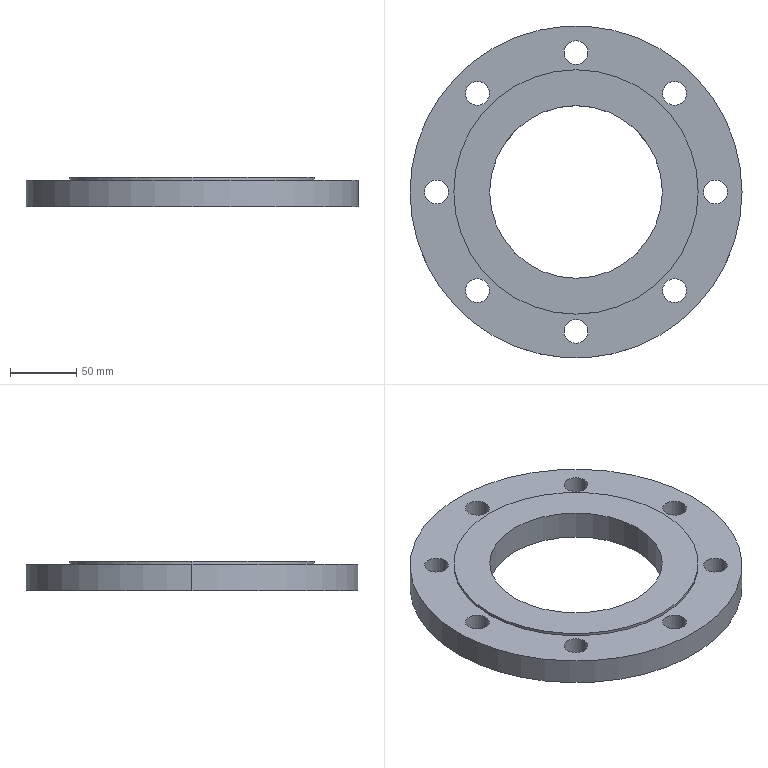Part | SolidWorks | features Extrusion 1, ICE 1 | 1 solid | 25 faces | box 250 x 250 x 22 mm | volume 702203 mm3 | cylinder 22 | plane 3 | commonest cylinder face diameters 18 x16 130 x2 184 x2 250 x2
STEP:
#1=CARTESIAN_POINT('',(92.,0.,22.));
#2=VERTEX_POINT('',#1);
#3=CARTESIAN_POINT('',(-92.,0.,22.));
#4=VERTEX_POINT('',#3);
#5=CARTESIAN_POINT('',(0.,0.,22.));
#6=DIRECTION('',(0.,0.,1.));
#7=DIRECTION('',(1.,0.,0.));
#8=AXIS2_PLACEMENT_3D('',#5,#6,#7);
#9=CIRCLE('',#8,92.);
#10=EDGE_CURVE('',#2,#4,#9,.T.);
#11=ORIENTED_EDGE('',*,*,#10,.F.);
#12=CARTESIAN_POINT('',(92.,0.,20.));
#13=VERTEX_POINT('',#12);
#14=CARTESIAN_POINT('',(92.,0.,22.));
#15=DIRECTION('',(0.,0.,-1.));
#16=VECTOR('',#15,1000.);
#17=LINE('',#14,#16);
#18=EDGE_CURVE('',#2,#13,#17,.T.);
#19=ORIENTED_EDGE('',*,*,#18,.T.);
#20=CARTESIAN_POINT('',(-92.,0.,20.));
#21=VERTEX_POINT('',#20);
#22=CARTESIAN_POINT('',(0.,0.,20.));
#23=DIRECTION('',(0.,0.,1.));
#24=DIRECTION('',(1.,0.,0.));
#25=AXIS2_PLACEMENT_3D('',#22,#23,#24);
#26=CIRCLE('',#25,92.);
#27=EDGE_CURVE('',#13,#21,#26,.T.);
#28=ORIENTED_EDGE('',*,*,#27,.T.);
#29=CARTESIAN_POINT('',(-92.,0.,22.));
#30=DIRECTION('',(0.,0.,-1.));
#31=VECTOR('',#30,1000.);
#32=LINE('',#29,#31);
#33=EDGE_CURVE('',#4,#21,#32,.T.);
#34=ORIENTED_EDGE('',*,*,#33,.F.);
#35=EDGE_LOOP('',(#11,#19,#28,#34));
#36=FACE_OUTER_BOUND('',#35,.T.);
#37=CARTESIAN_POINT('',(0.,0.,22.));
#38=DIRECTION('',(0.,0.,-1.));
#39=DIRECTION('',(-1.,0.,0.));
#40=AXIS2_PLACEMENT_3D('',#37,#38,#39);
#41=CYLINDRICAL_SURFACE('',#40,92.);
#42=ADVANCED_FACE('',(#36),#41,.T.);
#43=CARTESIAN_POINT('',(-83.246,74.246,20.));
#44=VERTEX_POINT('',#43);
#45=CARTESIAN_POINT('',(-65.246,74.246,20.));
#46=VERTEX_POINT('',#45);
#47=CARTESIAN_POINT('',(-74.246,74.246,20.));
#48=DIRECTION('',(0.,0.,1.));
#49=DIRECTION('',(1.,0.,0.));
#50=AXIS2_PLACEMENT_3D('',#47,#48,#49);
#51=CIRCLE('',#50,9.);
#52=EDGE_CURVE('',#44,#46,#51,.T.);
#53=ORIENTED_EDGE('',*,*,#52,.T.);
#54=CARTESIAN_POINT('',(-65.246,74.246,0.));
#55=VERTEX_POINT('',#54);
#56=CARTESIAN_POINT('',(-65.246,74.246,20.));
#57=DIRECTION('',(0.,0.,-1.));
#58=VECTOR('',#57,1000.);
#59=LINE('',#56,#58);
#60=EDGE_CURVE('',#46,#55,#59,.T.);
#61=ORIENTED_EDGE('',*,*,#60,.T.);
#62=CARTESIAN_POINT('',(-83.246,74.246,0.));
#63=VERTEX_POINT('',#62);
#64=CARTESIAN_POINT('',(-74.246,74.246,0.));
#65=DIRECTION('',(0.,0.,1.));
#66=DIRECTION('',(1.,0.,0.));
#67=AXIS2_PLACEMENT_3D('',#64,#65,#66);
#68=CIRCLE('',#67,9.);
#69=EDGE_CURVE('',#63,#55,#68,.T.);
#70=ORIENTED_EDGE('',*,*,#69,.F.);
#71=CARTESIAN_POINT('',(-83.246,74.246,20.));
#72=DIRECTION('',(0.,0.,-1.));
#73=VECTOR('',#72,1000.);
#74=LINE('',#71,#73);
#75=EDGE_CURVE('',#44,#63,#74,.T.);
#76=ORIENTED_EDGE('',*,*,#75,.F.);
#77=EDGE_LOOP('',(#53,#61,#70,#76));
#78=FACE_OUTER_BOUND('',#77,.T.);
#79=CARTESIAN_POINT('',(-74.246,74.246,20.));
#80=DIRECTION('',(0.,0.,-1.));
#81=DIRECTION('',(-1.,0.,0.));
#82=AXIS2_PLACEMENT_3D('',#79,#80,#81);
#83=CYLINDRICAL_SURFACE('',#82,9.);
#84=ADVANCED_FACE('',(#78),#83,.F.);
#85=CARTESIAN_POINT('',(-114.,0.,20.));
#86=VERTEX_POINT('',#85);
#87=CARTESIAN_POINT('',(-96.,0.,20.));
#88=VERTEX_POINT('',#87);
#89=CARTESIAN_POINT('',(-105.,0.,20.));
#90=DIRECTION('',(0.,0.,1.));
#91=DIRECTION('',(1.,0.,0.));
#92=AXIS2_PLACEMENT_3D('',#89,#90,#91);
#93=CIRCLE('',#92,9.);
#94=EDGE_CURVE('',#86,#88,#93,.T.);
#95=ORIENTED_EDGE('',*,*,#94,.T.);
#96=CARTESIAN_POINT('',(-96.,0.,0.));
#97=VERTEX_POINT('',#96);
#98=CARTESIAN_POINT('',(-96.,0.,20.));
#99=DIRECTION('',(0.,0.,-1.));
#100=VECTOR('',#99,1000.);
#101=LINE('',#98,#100);
#102=EDGE_CURVE('',#88,#97,#101,.T.);
#103=ORIENTED_EDGE('',*,*,#102,.T.);
#104=CARTESIAN_POINT('',(-114.,0.,0.));
#105=VERTEX_POINT('',#104);
#106=CARTESIAN_POINT('',(-105.,0.,0.));
#107=DIRECTION('',(0.,0.,1.));
#108=DIRECTION('',(1.,0.,0.));
#109=AXIS2_PLACEMENT_3D('',#106,#107,#108);
#110=CIRCLE('',#109,9.);
#111=EDGE_CURVE('',#105,#97,#110,.T.);
#112=ORIENTED_EDGE('',*,*,#111,.F.);
#113=CARTESIAN_POINT('',(-114.,0.,20.));
#114=DIRECTION('',(0.,0.,-1.));
#115=VECTOR('',#114,1000.);
#116=LINE('',#113,#115);
#117=EDGE_CURVE('',#86,#105,#116,.T.);
#118=ORIENTED_EDGE('',*,*,#117,.F.);
#119=EDGE_LOOP('',(#95,#103,#112,#118));
#120=FACE_OUTER_BOUND('',#119,.T.);
#121=CARTESIAN_POINT('',(-105.,0.,20.));
#122=DIRECTION('',(0.,0.,-1.));
#123=DIRECTION('',(-1.,0.,0.));
#124=AXIS2_PLACEMENT_3D('',#121,#122,#123);
#125=CYLINDRICAL_SURFACE('',#124,9.);
#126=ADVANCED_FACE('',(#120),#125,.F.);
#127=CARTESIAN_POINT('',(-83.246,-74.246,20.));
#128=VERTEX_POINT('',#127);
#129=CARTESIAN_POINT('',(-65.246,-74.246,20.));
#130=VERTEX_POINT('',#129);
#131=CARTESIAN_POINT('',(-74.246,-74.246,20.));
#132=DIRECTION('',(0.,0.,1.));
#133=DIRECTION('',(1.,0.,0.));
#134=AXIS2_PLACEMENT_3D('',#131,#132,#133);
#135=CIRCLE('',#134,9.);
#136=EDGE_CURVE('',#128,#130,#135,.T.);
#137=ORIENTED_EDGE('',*,*,#136,.T.);
#138=CARTESIAN_POINT('',(-65.246,-74.246,0.));
#139=VERTEX_POINT('',#138);
#140=CARTESIAN_POINT('',(-65.246,-74.246,20.));
#141=DIRECTION('',(0.,0.,-1.));
#142=VECTOR('',#141,1000.);
#143=LINE('',#140,#142);
#144=EDGE_CURVE('',#130,#139,#143,.T.);
#145=ORIENTED_EDGE('',*,*,#144,.T.);
#146=CARTESIAN_POINT('',(-83.246,-74.246,0.));
#147=VERTEX_POINT('',#146);
#148=CARTESIAN_POINT('',(-74.246,-74.246,0.));
#149=DIRECTION('',(0.,0.,1.));
#150=DIRECTION('',(1.,0.,0.));
#151=AXIS2_PLACEMENT_3D('',#148,#149,#150);
#152=CIRCLE('',#151,9.);
#153=EDGE_CURVE('',#147,#139,#152,.T.);
#154=ORIENTED_EDGE('',*,*,#153,.F.);
#155=CARTESIAN_POINT('',(-83.246,-74.246,20.));
#156=DIRECTION('',(0.,0.,-1.));
#157=VECTOR('',#156,1000.);
#158=LINE('',#155,#157);
#159=EDGE_CURVE('',#128,#147,#158,.T.);
#160=ORIENTED_EDGE('',*,*,#159,.F.);
#161=EDGE_LOOP('',(#137,#145,#154,#160));
#162=FACE_OUTER_BOUND('',#161,.T.);
#163=CARTESIAN_POINT('',(-74.246,-74.246,20.));
#164=DIRECTION('',(0.,0.,-1.));
#165=DIRECTION('',(-1.,0.,0.));
#166=AXIS2_PLACEMENT_3D('',#163,#164,#165);
#167=CYLINDRICAL_SURFACE('',#166,9.);
#168=ADVANCED_FACE('',(#162),#167,.F.);
#169=CARTESIAN_POINT('',(-9.,-105.,20.));
#170=VERTEX_POINT('',#169);
#171=CARTESIAN_POINT('',(9.,-105.,20.));
#172=VERTEX_POINT('',#171);
#173=CARTESIAN_POINT('',(0.,-105.,20.));
#174=DIRECTION('',(0.,0.,1.));
#175=DIRECTION('',(1.,0.,0.));
#176=AXIS2_PLACEMENT_3D('',#173,#174,#175);
#177=CIRCLE('',#176,9.);
#178=EDGE_CURVE('',#170,#172,#177,.T.);
#179=ORIENTED_EDGE('',*,*,#178,.T.);
#180=CARTESIAN_POINT('',(9.,-105.,0.));
#181=VERTEX_POINT('',#180);
#182=CARTESIAN_POINT('',(9.,-105.,20.));
#183=DIRECTION('',(0.,0.,-1.));
#184=VECTOR('',#183,1000.);
#185=LINE('',#182,#184);
#186=EDGE_CURVE('',#172,#181,#185,.T.);
#187=ORIENTED_EDGE('',*,*,#186,.T.);
#188=CARTESIAN_POINT('',(-9.,-105.,0.));
#189=VERTEX_POINT('',#188);
#190=CARTESIAN_POINT('',(0.,-105.,0.));
#191=DIRECTION('',(0.,0.,1.));
#192=DIRECTION('',(1.,0.,0.));
#193=AXIS2_PLACEMENT_3D('',#190,#191,#192);
#194=CIRCLE('',#193,9.);
#195=EDGE_CURVE('',#189,#181,#194,.T.);
#196=ORIENTED_EDGE('',*,*,#195,.F.);
#197=CARTESIAN_POINT('',(-9.,-105.,20.));
#198=DIRECTION('',(0.,0.,-1.));
#199=VECTOR('',#198,1000.);
#200=LINE('',#197,#199);
#201=EDGE_CURVE('',#170,#189,#200,.T.);
#202=ORIENTED_EDGE('',*,*,#201,.F.);
#203=EDGE_LOOP('',(#179,#187,#196,#202));
#204=FACE_OUTER_BOUND('',#203,.T.);
#205=CARTESIAN_POINT('',(0.,-105.,20.));
#206=DIRECTION('',(0.,0.,-1.));
#207=DIRECTION('',(-1.,0.,0.));
#208=AXIS2_PLACEMENT_3D('',#205,#206,#207);
#209=CYLINDRICAL_SURFACE('',#208,9.);
#210=ADVANCED_FACE('',(#204),#209,.F.);
#211=CARTESIAN_POINT('',(65.246,-74.246,20.));
#212=VERTEX_POINT('',#211);
#213=CARTESIAN_POINT('',(83.246,-74.246,20.));
#214=VERTEX_POINT('',#213);
#215=CARTESIAN_POINT('',(74.246,-74.246,20.));
#216=DIRECTION('',(0.,0.,1.));
#217=DIRECTION('',(1.,0.,0.));
#218=AXIS2_PLACEMENT_3D('',#215,#216,#217);
#219=CIRCLE('',#218,9.);
#220=EDGE_CURVE('',#212,#214,#219,.T.);
#221=ORIENTED_EDGE('',*,*,#220,.T.);
#222=CARTESIAN_POINT('',(83.246,-74.246,0.));
#223=VERTEX_POINT('',#222);
#224=CARTESIAN_POINT('',(83.246,-74.246,20.));
#225=DIRECTION('',(0.,0.,-1.));
#226=VECTOR('',#225,1000.);
#227=LINE('',#224,#226);
#228=EDGE_CURVE('',#214,#223,#227,.T.);
#229=ORIENTED_EDGE('',*,*,#228,.T.);
#230=CARTESIAN_POINT('',(65.246,-74.246,0.));
#231=VERTEX_POINT('',#230);
#232=CARTESIAN_POINT('',(74.246,-74.246,0.));
#233=DIRECTION('',(0.,0.,1.));
#234=DIRECTION('',(1.,0.,0.));
#235=AXIS2_PLACEMENT_3D('',#232,#233,#234);
#236=CIRCLE('',#235,9.);
#237=EDGE_CURVE('',#231,#223,#236,.T.);
#238=ORIENTED_EDGE('',*,*,#237,.F.);
#239=CARTESIAN_POINT('',(65.246,-74.246,20.));
#240=DIRECTION('',(0.,0.,-1.));
#241=VECTOR('',#240,1000.);
#242=LINE('',#239,#241);
#243=EDGE_CURVE('',#212,#231,#242,.T.);
#244=ORIENTED_EDGE('',*,*,#243,.F.);
#245=EDGE_LOOP('',(#221,#229,#238,#244));
#246=FACE_OUTER_BOUND('',#245,.T.);
#247=CARTESIAN_POINT('',(74.246,-74.246,20.));
#248=DIRECTION('',(0.,0.,-1.));
#249=DIRECTION('',(-1.,0.,0.));
#250=AXIS2_PLACEMENT_3D('',#247,#248,#249);
#251=CYLINDRICAL_SURFACE('',#250,9.);
#252=ADVANCED_FACE('',(#246),#251,.F.);
#253=CARTESIAN_POINT('',(96.,0.,20.));
#254=VERTEX_POINT('',#253);
#255=CARTESIAN_POINT('',(114.,0.,20.));
#256=VERTEX_POINT('',#255);
#257=CARTESIAN_POINT('',(105.,0.,20.));
#258=DIRECTION('',(0.,0.,1.));
#259=DIRECTION('',(1.,0.,0.));
#260=AXIS2_PLACEMENT_3D('',#257,#258,#259);
#261=CIRCLE('',#260,9.);
#262=EDGE_CURVE('',#254,#256,#261,.T.);
#263=ORIENTED_EDGE('',*,*,#262,.T.);
#264=CARTESIAN_POINT('',(114.,0.,0.));
#265=VERTEX_POINT('',#264);
#266=CARTESIAN_POINT('',(114.,0.,20.));
#267=DIRECTION('',(0.,0.,-1.));
#268=VECTOR('',#267,1000.);
#269=LINE('',#266,#268);
#270=EDGE_CURVE('',#256,#265,#269,.T.);
#271=ORIENTED_EDGE('',*,*,#270,.T.);
#272=CARTESIAN_POINT('',(96.,0.,0.));
#273=VERTEX_POINT('',#272);
#274=CARTESIAN_POINT('',(105.,0.,0.));
#275=DIRECTION('',(0.,0.,1.));
#276=DIRECTION('',(1.,0.,0.));
#277=AXIS2_PLACEMENT_3D('',#274,#275,#276);
#278=CIRCLE('',#277,9.);
#279=EDGE_CURVE('',#273,#265,#278,.T.);
#280=ORIENTED_EDGE('',*,*,#279,.F.);
#281=CARTESIAN_POINT('',(96.,0.,20.));
#282=DIRECTION('',(0.,0.,-1.));
#283=VECTOR('',#282,1000.);
#284=LINE('',#281,#283);
#285=EDGE_CURVE('',#254,#273,#284,.T.);
#286=ORIENTED_EDGE('',*,*,#285,.F.);
#287=EDGE_LOOP('',(#263,#271,#280,#286));
#288=FACE_OUTER_BOUND('',#287,.T.);
#289=CARTESIAN_POINT('',(105.,0.,20.));
#290=DIRECTION('',(0.,0.,-1.));
#291=DIRECTION('',(-1.,0.,0.));
#292=AXIS2_PLACEMENT_3D('',#289,#290,#291);
#293=CYLINDRICAL_SURFACE('',#292,9.);
#294=ADVANCED_FACE('',(#288),#293,.F.);
#295=CARTESIAN_POINT('',(65.246,74.246,20.));
#296=VERTEX_POINT('',#295);
#297=CARTESIAN_POINT('',(83.246,74.246,20.));
#298=VERTEX_POINT('',#297);
#299=CARTESIAN_POINT('',(74.246,74.246,20.));
#300=DIRECTION('',(0.,0.,1.));
#301=DIRECTION('',(1.,0.,0.));
#302=AXIS2_PLACEMENT_3D('',#299,#300,#301);
#303=CIRCLE('',#302,9.);
#304=EDGE_CURVE('',#296,#298,#303,.T.);
#305=ORIENTED_EDGE('',*,*,#304,.T.);
#306=CARTESIAN_POINT('',(83.246,74.246,0.));
#307=VERTEX_POINT('',#306);
#308=CARTESIAN_POINT('',(83.246,74.246,20.));
#309=DIRECTION('',(0.,0.,-1.));
#310=VECTOR('',#309,1000.);
#311=LINE('',#308,#310);
#312=EDGE_CURVE('',#298,#307,#311,.T.);
#313=ORIENTED_EDGE('',*,*,#312,.T.);
#314=CARTESIAN_POINT('',(65.246,74.246,0.));
#315=VERTEX_POINT('',#314);
#316=CARTESIAN_POINT('',(74.246,74.246,0.));
#317=DIRECTION('',(0.,0.,1.));
#318=DIRECTION('',(1.,0.,0.));
#319=AXIS2_PLACEMENT_3D('',#316,#317,#318);
#320=CIRCLE('',#319,9.);
#321=EDGE_CURVE('',#315,#307,#320,.T.);
#322=ORIENTED_EDGE('',*,*,#321,.F.);
#323=CARTESIAN_POINT('',(65.246,74.246,20.));
#324=DIRECTION('',(0.,0.,-1.));
#325=VECTOR('',#324,1000.);
#326=LINE('',#323,#325);
#327=EDGE_CURVE('',#296,#315,#326,.T.);
#328=ORIENTED_EDGE('',*,*,#327,.F.);
#329=EDGE_LOOP('',(#305,#313,#322,#328));
#330=FACE_OUTER_BOUND('',#329,.T.);
#331=CARTESIAN_POINT('',(74.246,74.246,20.));
#332=DIRECTION('',(0.,0.,-1.));
#333=DIRECTION('',(-1.,0.,0.));
#334=AXIS2_PLACEMENT_3D('',#331,#332,#333);
#335=CYLINDRICAL_SURFACE('',#334,9.);
#336=ADVANCED_FACE('',(#330),#335,.F.);
#337=CARTESIAN_POINT('',(-9.,105.,20.));
#338=VERTEX_POINT('',#337);
#339=CARTESIAN_POINT('',(9.,105.,20.));
#340=VERTEX_POINT('',#339);
#341=CARTESIAN_POINT('',(0.,105.,20.));
#342=DIRECTION('',(0.,0.,1.));
#343=DIRECTION('',(1.,0.,0.));
#344=AXIS2_PLACEMENT_3D('',#341,#342,#343);
#345=CIRCLE('',#344,9.);
#346=EDGE_CURVE('',#338,#340,#345,.T.);
#347=ORIENTED_EDGE('',*,*,#346,.T.);
#348=CARTESIAN_POINT('',(9.,105.,0.));
#349=VERTEX_POINT('',#348);
#350=CARTESIAN_POINT('',(9.,105.,20.));
#351=DIRECTION('',(0.,0.,-1.));
#352=VECTOR('',#351,1000.);
#353=LINE('',#350,#352);
#354=EDGE_CURVE('',#340,#349,#353,.T.);
#355=ORIENTED_EDGE('',*,*,#354,.T.);
#356=CARTESIAN_POINT('',(-9.,105.,0.));
#357=VERTEX_POINT('',#356);
#358=CARTESIAN_POINT('',(0.,105.,0.));
#359=DIRECTION('',(0.,0.,1.));
#360=DIRECTION('',(1.,0.,0.));
#361=AXIS2_PLACEMENT_3D('',#358,#359,#360);
#362=CIRCLE('',#361,9.);
#363=EDGE_CURVE('',#357,#349,#362,.T.);
#364=ORIENTED_EDGE('',*,*,#363,.F.);
#365=CARTESIAN_POINT('',(-9.,105.,20.));
#366=DIRECTION('',(0.,0.,-1.));
#367=VECTOR('',#366,1000.);
#368=LINE('',#365,#367);
#369=EDGE_CURVE('',#338,#357,#368,.T.);
#370=ORIENTED_EDGE('',*,*,#369,.F.);
#371=EDGE_LOOP('',(#347,#355,#364,#370));
#372=FACE_OUTER_BOUND('',#371,.T.);
#373=CARTESIAN_POINT('',(0.,105.,20.));
#374=DIRECTION('',(0.,0.,-1.));
#375=DIRECTION('',(-1.,0.,0.));
#376=AXIS2_PLACEMENT_3D('',#373,#374,#375);
#377=CYLINDRICAL_SURFACE('',#376,9.);
#378=ADVANCED_FACE('',(#372),#377,.F.);
#379=CARTESIAN_POINT('',(-65.,0.,22.));
#380=VERTEX_POINT('',#379);
#381=CARTESIAN_POINT('',(65.,0.,22.));
#382=VERTEX_POINT('',#381);
#383=CARTESIAN_POINT('',(0.,0.,22.));
#384=DIRECTION('',(0.,0.,1.));
#385=DIRECTION('',(1.,0.,0.));
#386=AXIS2_PLACEMENT_3D('',#383,#384,#385);
#387=CIRCLE('',#386,65.);
#388=EDGE_CURVE('',#380,#382,#387,.T.);
#389=ORIENTED_EDGE('',*,*,#388,.T.);
#390=CARTESIAN_POINT('',(65.,0.,0.));
#391=VERTEX_POINT('',#390);
#392=CARTESIAN_POINT('',(65.,0.,20.));
#393=DIRECTION('',(0.,0.,-1.));
#394=VECTOR('',#393,1000.);
#395=LINE('',#392,#394);
#396=EDGE_CURVE('',#382,#391,#395,.T.);
#397=ORIENTED_EDGE('',*,*,#396,.T.);
#398=CARTESIAN_POINT('',(-65.,0.,0.));
#399=VERTEX_POINT('',#398);
#400=CARTESIAN_POINT('',(0.,0.,0.));
#401=DIRECTION('',(0.,0.,1.));
#402=DIRECTION('',(1.,0.,0.));
#403=AXIS2_PLACEMENT_3D('',#400,#401,#402);
#404=CIRCLE('',#403,65.);
#405=EDGE_CURVE('',#399,#391,#404,.T.);
#406=ORIENTED_EDGE('',*,*,#405,.F.);
#407=CARTESIAN_POINT('',(-65.,0.,20.));
#408=DIRECTION('',(0.,0.,-1.));
#409=VECTOR('',#408,1000.);
#410=LINE('',#407,#409);
#411=EDGE_CURVE('',#380,#399,#410,.T.);
#412=ORIENTED_EDGE('',*,*,#411,.F.);
#413=EDGE_LOOP('',(#389,#397,#406,#412));
#414=FACE_OUTER_BOUND('',#413,.T.);
#415=CARTESIAN_POINT('',(0.,0.,20.));
#416=DIRECTION('',(0.,0.,-1.));
#417=DIRECTION('',(-1.,0.,0.));
#418=AXIS2_PLACEMENT_3D('',#415,#416,#417);
#419=CYLINDRICAL_SURFACE('',#418,65.);
#420=ADVANCED_FACE('',(#414),#419,.F.);
#421=CARTESIAN_POINT('',(125.,0.,20.));
#422=VERTEX_POINT('',#421);
#423=CARTESIAN_POINT('',(-125.,0.,20.));
#424=VERTEX_POINT('',#423);
#425=CARTESIAN_POINT('',(0.,0.,20.));
#426=DIRECTION('',(0.,0.,1.));
#427=DIRECTION('',(1.,0.,0.));
#428=AXIS2_PLACEMENT_3D('',#425,#426,#427);
#429=CIRCLE('',#428,125.);
#430=EDGE_CURVE('',#422,#424,#429,.T.);
#431=ORIENTED_EDGE('',*,*,#430,.F.);
#432=CARTESIAN_POINT('',(125.,0.,0.));
#433=VERTEX_POINT('',#432);
#434=CARTESIAN_POINT('',(125.,0.,20.));
#435=DIRECTION('',(0.,0.,-1.));
#436=VECTOR('',#435,1000.);
#437=LINE('',#434,#436);
#438=EDGE_CURVE('',#422,#433,#437,.T.);
#439=ORIENTED_EDGE('',*,*,#438,.T.);
#440=CARTESIAN_POINT('',(-125.,0.,0.));
#441=VERTEX_POINT('',#440);
#442=CARTESIAN_POINT('',(0.,0.,0.));
#443=DIRECTION('',(0.,0.,1.));
#444=DIRECTION('',(1.,0.,0.));
#445=AXIS2_PLACEMENT_3D('',#442,#443,#444);
#446=CIRCLE('',#445,125.);
#447=EDGE_CURVE('',#433,#441,#446,.T.);
#448=ORIENTED_EDGE('',*,*,#447,.T.);
#449=CARTESIAN_POINT('',(-125.,0.,20.));
#450=DIRECTION('',(0.,0.,-1.));
#451=VECTOR('',#450,1000.);
#452=LINE('',#449,#451);
#453=EDGE_CURVE('',#424,#441,#452,.T.);
#454=ORIENTED_EDGE('',*,*,#453,.F.);
#455=EDGE_LOOP('',(#431,#439,#448,#454));
#456=FACE_OUTER_BOUND('',#455,.T.);
#457=CARTESIAN_POINT('',(0.,0.,20.));
#458=DIRECTION('',(0.,0.,-1.));
#459=DIRECTION('',(-1.,0.,0.));
#460=AXIS2_PLACEMENT_3D('',#457,#458,#459);
#461=CYLINDRICAL_SURFACE('',#460,125.);
#462=ADVANCED_FACE('',(#456),#461,.T.);
#463=ORIENTED_EDGE('',*,*,#52,.F.);
#464=CARTESIAN_POINT('',(-74.246,74.246,20.));
#465=DIRECTION('',(0.,0.,1.));
#466=DIRECTION('',(1.,0.,0.));
#467=AXIS2_PLACEMENT_3D('',#464,#465,#466);
#468=CIRCLE('',#467,9.);
#469=EDGE_CURVE('',#46,#44,#468,.T.);
#470=ORIENTED_EDGE('',*,*,#469,.F.);
#471=EDGE_LOOP('',(#463,#470));
#472=FACE_BOUND('',#471,.T.);
#473=ORIENTED_EDGE('',*,*,#136,.F.);
#474=CARTESIAN_POINT('',(-74.246,-74.246,20.));
#475=DIRECTION('',(0.,0.,1.));
#476=DIRECTION('',(1.,0.,0.));
#477=AXIS2_PLACEMENT_3D('',#474,#475,#476);
#478=CIRCLE('',#477,9.);
#479=EDGE_CURVE('',#130,#128,#478,.T.);
#480=ORIENTED_EDGE('',*,*,#479,.F.);
#481=EDGE_LOOP('',(#473,#480));
#482=FACE_BOUND('',#481,.T.);
#483=ORIENTED_EDGE('',*,*,#220,.F.);
#484=CARTESIAN_POINT('',(74.246,-74.246,20.));
#485=DIRECTION('',(0.,0.,1.));
#486=DIRECTION('',(1.,0.,0.));
#487=AXIS2_PLACEMENT_3D('',#484,#485,#486);
#488=CIRCLE('',#487,9.);
#489=EDGE_CURVE('',#214,#212,#488,.T.);
#490=ORIENTED_EDGE('',*,*,#489,.F.);
#491=EDGE_LOOP('',(#483,#490));
#492=FACE_BOUND('',#491,.T.);
#493=ORIENTED_EDGE('',*,*,#304,.F.);
#494=CARTESIAN_POINT('',(74.246,74.246,20.));
#495=DIRECTION('',(0.,0.,1.));
#496=DIRECTION('',(1.,0.,0.));
#497=AXIS2_PLACEMENT_3D('',#494,#495,#496);
#498=CIRCLE('',#497,9.);
#499=EDGE_CURVE('',#298,#296,#498,.T.);
#500=ORIENTED_EDGE('',*,*,#499,.F.);
#501=EDGE_LOOP('',(#493,#500));
#502=FACE_BOUND('',#501,.T.);
#503=CARTESIAN_POINT('',(0.,0.,20.));
#504=DIRECTION('',(0.,0.,1.));
#505=DIRECTION('',(1.,0.,0.));
#506=AXIS2_PLACEMENT_3D('',#503,#504,#505);
#507=CIRCLE('',#506,125.);
#508=EDGE_CURVE('',#424,#422,#507,.T.);
#509=ORIENTED_EDGE('',*,*,#508,.T.);
#510=ORIENTED_EDGE('',*,*,#430,.T.);
#511=EDGE_LOOP('',(#509,#510));
#512=FACE_OUTER_BOUND('',#511,.T.);
#513=ORIENTED_EDGE('',*,*,#346,.F.);
#514=CARTESIAN_POINT('',(0.,105.,20.));
#515=DIRECTION('',(0.,0.,1.));
#516=DIRECTION('',(1.,0.,0.));
#517=AXIS2_PLACEMENT_3D('',#514,#515,#516);
#518=CIRCLE('',#517,9.);
#519=EDGE_CURVE('',#340,#338,#518,.T.);
#520=ORIENTED_EDGE('',*,*,#519,.F.);
#521=EDGE_LOOP('',(#513,#520));
#522=FACE_BOUND('',#521,.T.);
#523=ORIENTED_EDGE('',*,*,#262,.F.);
#524=CARTESIAN_POINT('',(105.,0.,20.));
#525=DIRECTION('',(0.,0.,1.));
#526=DIRECTION('',(1.,0.,0.));
#527=AXIS2_PLACEMENT_3D('',#524,#525,#526);
#528=CIRCLE('',#527,9.);
#529=EDGE_CURVE('',#256,#254,#528,.T.);
#530=ORIENTED_EDGE('',*,*,#529,.F.);
#531=EDGE_LOOP('',(#523,#530));
#532=FACE_BOUND('',#531,.T.);
#533=ORIENTED_EDGE('',*,*,#178,.F.);
#534=CARTESIAN_POINT('',(0.,-105.,20.));
#535=DIRECTION('',(0.,0.,1.));
#536=DIRECTION('',(1.,0.,0.));
#537=AXIS2_PLACEMENT_3D('',#534,#535,#536);
#538=CIRCLE('',#537,9.);
#539=EDGE_CURVE('',#172,#170,#538,.T.);
#540=ORIENTED_EDGE('',*,*,#539,.F.);
#541=EDGE_LOOP('',(#533,#540));
#542=FACE_BOUND('',#541,.T.);
#543=ORIENTED_EDGE('',*,*,#94,.F.);
#544=CARTESIAN_POINT('',(-105.,0.,20.));
#545=DIRECTION('',(0.,0.,1.));
#546=DIRECTION('',(1.,0.,0.));
#547=AXIS2_PLACEMENT_3D('',#544,#545,#546);
#548=CIRCLE('',#547,9.);
#549=EDGE_CURVE('',#88,#86,#548,.T.);
#550=ORIENTED_EDGE('',*,*,#549,.F.);
#551=EDGE_LOOP('',(#543,#550));
#552=FACE_BOUND('',#551,.T.);
#553=CARTESIAN_POINT('',(0.,0.,20.));
#554=DIRECTION('',(0.,0.,1.));
#555=DIRECTION('',(1.,0.,0.));
#556=AXIS2_PLACEMENT_3D('',#553,#554,#555);
#557=CIRCLE('',#556,92.);
#558=EDGE_CURVE('',#21,#13,#557,.T.);
#559=ORIENTED_EDGE('',*,*,#558,.F.);
#560=ORIENTED_EDGE('',*,*,#27,.F.);
#561=EDGE_LOOP('',(#559,#560));
#562=FACE_BOUND('',#561,.T.);
#563=CARTESIAN_POINT('',(0.,0.,20.));
#564=DIRECTION('',(0.,0.,1.));
#565=DIRECTION('',(1.,0.,0.));
#566=AXIS2_PLACEMENT_3D('',#563,#564,#565);
#567=PLANE('',#566);
#568=ADVANCED_FACE('',(#472,#482,#492,#502,#512,#522,#532,#542,#552,#562),#567,.T.);
#569=CARTESIAN_POINT('',(0.,0.,0.));
#570=DIRECTION('',(0.,0.,1.));
#571=DIRECTION('',(1.,0.,0.));
#572=AXIS2_PLACEMENT_3D('',#569,#570,#571);
#573=CIRCLE('',#572,125.);
#574=EDGE_CURVE('',#441,#433,#573,.T.);
#575=ORIENTED_EDGE('',*,*,#574,.F.);
#576=ORIENTED_EDGE('',*,*,#447,.F.);
#577=EDGE_LOOP('',(#575,#576));
#578=FACE_OUTER_BOUND('',#577,.T.);
#579=ORIENTED_EDGE('',*,*,#405,.T.);
#580=CARTESIAN_POINT('',(0.,0.,0.));
#581=DIRECTION('',(0.,0.,1.));
#582=DIRECTION('',(1.,0.,0.));
#583=AXIS2_PLACEMENT_3D('',#580,#581,#582);
#584=CIRCLE('',#583,65.);
#585=EDGE_CURVE('',#391,#399,#584,.T.);
#586=ORIENTED_EDGE('',*,*,#585,.T.);
#587=EDGE_LOOP('',(#579,#586));
#588=FACE_BOUND('',#587,.T.);
#589=ORIENTED_EDGE('',*,*,#363,.T.);
#590=CARTESIAN_POINT('',(0.,105.,0.));
#591=DIRECTION('',(0.,0.,1.));
#592=DIRECTION('',(1.,0.,0.));
#593=AXIS2_PLACEMENT_3D('',#590,#591,#592);
#594=CIRCLE('',#593,9.);
#595=EDGE_CURVE('',#349,#357,#594,.T.);
#596=ORIENTED_EDGE('',*,*,#595,.T.);
#597=EDGE_LOOP('',(#589,#596));
#598=FACE_BOUND('',#597,.T.);
#599=ORIENTED_EDGE('',*,*,#321,.T.);
#600=CARTESIAN_POINT('',(74.246,74.246,0.));
#601=DIRECTION('',(0.,0.,1.));
#602=DIRECTION('',(1.,0.,0.));
#603=AXIS2_PLACEMENT_3D('',#600,#601,#602);
#604=CIRCLE('',#603,9.);
#605=EDGE_CURVE('',#307,#315,#604,.T.);
#606=ORIENTED_EDGE('',*,*,#605,.T.);
#607=EDGE_LOOP('',(#599,#606));
#608=FACE_BOUND('',#607,.T.);
#609=ORIENTED_EDGE('',*,*,#279,.T.);
#610=CARTESIAN_POINT('',(105.,0.,0.));
#611=DIRECTION('',(0.,0.,1.));
#612=DIRECTION('',(1.,0.,0.));
#613=AXIS2_PLACEMENT_3D('',#610,#611,#612);
#614=CIRCLE('',#613,9.);
#615=EDGE_CURVE('',#265,#273,#614,.T.);
#616=ORIENTED_EDGE('',*,*,#615,.T.);
#617=EDGE_LOOP('',(#609,#616));
#618=FACE_BOUND('',#617,.T.);
#619=ORIENTED_EDGE('',*,*,#237,.T.);
#620=CARTESIAN_POINT('',(74.246,-74.246,0.));
#621=DIRECTION('',(0.,0.,1.));
#622=DIRECTION('',(1.,0.,0.));
#623=AXIS2_PLACEMENT_3D('',#620,#621,#622);
#624=CIRCLE('',#623,9.);
#625=EDGE_CURVE('',#223,#231,#624,.T.);
#626=ORIENTED_EDGE('',*,*,#625,.T.);
#627=EDGE_LOOP('',(#619,#626));
#628=FACE_BOUND('',#627,.T.);
#629=ORIENTED_EDGE('',*,*,#195,.T.);
#630=CARTESIAN_POINT('',(0.,-105.,0.));
#631=DIRECTION('',(0.,0.,1.));
#632=DIRECTION('',(1.,0.,0.));
#633=AXIS2_PLACEMENT_3D('',#630,#631,#632);
#634=CIRCLE('',#633,9.);
#635=EDGE_CURVE('',#181,#189,#634,.T.);
#636=ORIENTED_EDGE('',*,*,#635,.T.);
#637=EDGE_LOOP('',(#629,#636));
#638=FACE_BOUND('',#637,.T.);
#639=ORIENTED_EDGE('',*,*,#153,.T.);
#640=CARTESIAN_POINT('',(-74.246,-74.246,0.));
#641=DIRECTION('',(0.,0.,1.));
#642=DIRECTION('',(1.,0.,0.));
#643=AXIS2_PLACEMENT_3D('',#640,#641,#642);
#644=CIRCLE('',#643,9.);
#645=EDGE_CURVE('',#139,#147,#644,.T.);
#646=ORIENTED_EDGE('',*,*,#645,.T.);
#647=EDGE_LOOP('',(#639,#646));
#648=FACE_BOUND('',#647,.T.);
#649=ORIENTED_EDGE('',*,*,#111,.T.);
#650=CARTESIAN_POINT('',(-105.,0.,0.));
#651=DIRECTION('',(0.,0.,1.));
#652=DIRECTION('',(1.,0.,0.));
#653=AXIS2_PLACEMENT_3D('',#650,#651,#652);
#654=CIRCLE('',#653,9.);
#655=EDGE_CURVE('',#97,#105,#654,.T.);
#656=ORIENTED_EDGE('',*,*,#655,.T.);
#657=EDGE_LOOP('',(#649,#656));
#658=FACE_BOUND('',#657,.T.);
#659=ORIENTED_EDGE('',*,*,#69,.T.);
#660=CARTESIAN_POINT('',(-74.246,74.246,0.));
#661=DIRECTION('',(0.,0.,1.));
#662=DIRECTION('',(1.,0.,0.));
#663=AXIS2_PLACEMENT_3D('',#660,#661,#662);
#664=CIRCLE('',#663,9.);
#665=EDGE_CURVE('',#55,#63,#664,.T.);
#666=ORIENTED_EDGE('',*,*,#665,.T.);
#667=EDGE_LOOP('',(#659,#666));
#668=FACE_BOUND('',#667,.T.);
#669=CARTESIAN_POINT('',(0.,0.,0.));
#670=DIRECTION('',(0.,0.,1.));
#671=DIRECTION('',(1.,0.,0.));
#672=AXIS2_PLACEMENT_3D('',#669,#670,#671);
#673=PLANE('',#672);
#674=ADVANCED_FACE('',(#578,#588,#598,#608,#618,#628,#638,#648,#658,#668),#673,.F.);
#675=ORIENTED_EDGE('',*,*,#438,.F.);
#676=ORIENTED_EDGE('',*,*,#508,.F.);
#677=ORIENTED_EDGE('',*,*,#453,.T.);
#678=ORIENTED_EDGE('',*,*,#574,.T.);
#679=EDGE_LOOP('',(#675,#676,#677,#678));
#680=FACE_OUTER_BOUND('',#679,.T.);
#681=CARTESIAN_POINT('',(0.,0.,20.));
#682=DIRECTION('',(0.,0.,-1.));
#683=DIRECTION('',(-1.,0.,0.));
#684=AXIS2_PLACEMENT_3D('',#681,#682,#683);
#685=CYLINDRICAL_SURFACE('',#684,125.);
#686=ADVANCED_FACE('',(#680),#685,.T.);
#687=ORIENTED_EDGE('',*,*,#396,.F.);
#688=CARTESIAN_POINT('',(0.,0.,22.));
#689=DIRECTION('',(0.,0.,1.));
#690=DIRECTION('',(1.,0.,0.));
#691=AXIS2_PLACEMENT_3D('',#688,#689,#690);
#692=CIRCLE('',#691,65.);
#693=EDGE_CURVE('',#382,#380,#692,.T.);
#694=ORIENTED_EDGE('',*,*,#693,.T.);
#695=ORIENTED_EDGE('',*,*,#411,.T.);
#696=ORIENTED_EDGE('',*,*,#585,.F.);
#697=EDGE_LOOP('',(#687,#694,#695,#696));
#698=FACE_OUTER_BOUND('',#697,.T.);
#699=CARTESIAN_POINT('',(0.,0.,20.));
#700=DIRECTION('',(0.,0.,-1.));
#701=DIRECTION('',(-1.,0.,0.));
#702=AXIS2_PLACEMENT_3D('',#699,#700,#701);
#703=CYLINDRICAL_SURFACE('',#702,65.);
#704=ADVANCED_FACE('',(#698),#703,.F.);
#705=ORIENTED_EDGE('',*,*,#354,.F.);
#706=ORIENTED_EDGE('',*,*,#519,.T.);
#707=ORIENTED_EDGE('',*,*,#369,.T.);
#708=ORIENTED_EDGE('',*,*,#595,.F.);
#709=EDGE_LOOP('',(#705,#706,#707,#708));
#710=FACE_OUTER_BOUND('',#709,.T.);
#711=CARTESIAN_POINT('',(0.,105.,20.));
#712=DIRECTION('',(0.,0.,-1.));
#713=DIRECTION('',(-1.,0.,0.));
#714=AXIS2_PLACEMENT_3D('',#711,#712,#713);
#715=CYLINDRICAL_SURFACE('',#714,9.);
#716=ADVANCED_FACE('',(#710),#715,.F.);
#717=ORIENTED_EDGE('',*,*,#312,.F.);
#718=ORIENTED_EDGE('',*,*,#499,.T.);
#719=ORIENTED_EDGE('',*,*,#327,.T.);
#720=ORIENTED_EDGE('',*,*,#605,.F.);
#721=EDGE_LOOP('',(#717,#718,#719,#720));
#722=FACE_OUTER_BOUND('',#721,.T.);
#723=CARTESIAN_POINT('',(74.246,74.246,20.));
#724=DIRECTION('',(0.,0.,-1.));
#725=DIRECTION('',(-1.,0.,0.));
#726=AXIS2_PLACEMENT_3D('',#723,#724,#725);
#727=CYLINDRICAL_SURFACE('',#726,9.);
#728=ADVANCED_FACE('',(#722),#727,.F.);
#729=ORIENTED_EDGE('',*,*,#270,.F.);
#730=ORIENTED_EDGE('',*,*,#529,.T.);
#731=ORIENTED_EDGE('',*,*,#285,.T.);
#732=ORIENTED_EDGE('',*,*,#615,.F.);
#733=EDGE_LOOP('',(#729,#730,#731,#732));
#734=FACE_OUTER_BOUND('',#733,.T.);
#735=CARTESIAN_POINT('',(105.,0.,20.));
#736=DIRECTION('',(0.,0.,-1.));
#737=DIRECTION('',(-1.,0.,0.));
#738=AXIS2_PLACEMENT_3D('',#735,#736,#737);
#739=CYLINDRICAL_SURFACE('',#738,9.);
#740=ADVANCED_FACE('',(#734),#739,.F.);
#741=ORIENTED_EDGE('',*,*,#228,.F.);
#742=ORIENTED_EDGE('',*,*,#489,.T.);
#743=ORIENTED_EDGE('',*,*,#243,.T.);
#744=ORIENTED_EDGE('',*,*,#625,.F.);
#745=EDGE_LOOP('',(#741,#742,#743,#744));
#746=FACE_OUTER_BOUND('',#745,.T.);
#747=CARTESIAN_POINT('',(74.246,-74.246,20.));
#748=DIRECTION('',(0.,0.,-1.));
#749=DIRECTION('',(-1.,0.,0.));
#750=AXIS2_PLACEMENT_3D('',#747,#748,#749);
#751=CYLINDRICAL_SURFACE('',#750,9.);
#752=ADVANCED_FACE('',(#746),#751,.F.);
#753=ORIENTED_EDGE('',*,*,#186,.F.);
#754=ORIENTED_EDGE('',*,*,#539,.T.);
#755=ORIENTED_EDGE('',*,*,#201,.T.);
#756=ORIENTED_EDGE('',*,*,#635,.F.);
#757=EDGE_LOOP('',(#753,#754,#755,#756));
#758=FACE_OUTER_BOUND('',#757,.T.);
#759=CARTESIAN_POINT('',(0.,-105.,20.));
#760=DIRECTION('',(0.,0.,-1.));
#761=DIRECTION('',(-1.,0.,0.));
#762=AXIS2_PLACEMENT_3D('',#759,#760,#761);
#763=CYLINDRICAL_SURFACE('',#762,9.);
#764=ADVANCED_FACE('',(#758),#763,.F.);
#765=ORIENTED_EDGE('',*,*,#144,.F.);
#766=ORIENTED_EDGE('',*,*,#479,.T.);
#767=ORIENTED_EDGE('',*,*,#159,.T.);
#768=ORIENTED_EDGE('',*,*,#645,.F.);
#769=EDGE_LOOP('',(#765,#766,#767,#768));
#770=FACE_OUTER_BOUND('',#769,.T.);
#771=CARTESIAN_POINT('',(-74.246,-74.246,20.));
#772=DIRECTION('',(0.,0.,-1.));
#773=DIRECTION('',(-1.,0.,0.));
#774=AXIS2_PLACEMENT_3D('',#771,#772,#773);
#775=CYLINDRICAL_SURFACE('',#774,9.);
#776=ADVANCED_FACE('',(#770),#775,.F.);
#777=ORIENTED_EDGE('',*,*,#102,.F.);
#778=ORIENTED_EDGE('',*,*,#549,.T.);
#779=ORIENTED_EDGE('',*,*,#117,.T.);
#780=ORIENTED_EDGE('',*,*,#655,.F.);
#781=EDGE_LOOP('',(#777,#778,#779,#780));
#782=FACE_OUTER_BOUND('',#781,.T.);
#783=CARTESIAN_POINT('',(-105.,0.,20.));
#784=DIRECTION('',(0.,0.,-1.));
#785=DIRECTION('',(-1.,0.,0.));
#786=AXIS2_PLACEMENT_3D('',#783,#784,#785);
#787=CYLINDRICAL_SURFACE('',#786,9.);
#788=ADVANCED_FACE('',(#782),#787,.F.);
#789=ORIENTED_EDGE('',*,*,#60,.F.);
#790=ORIENTED_EDGE('',*,*,#469,.T.);
#791=ORIENTED_EDGE('',*,*,#75,.T.);
#792=ORIENTED_EDGE('',*,*,#665,.F.);
#793=EDGE_LOOP('',(#789,#790,#791,#792));
#794=FACE_OUTER_BOUND('',#793,.T.);
#795=CARTESIAN_POINT('',(-74.246,74.246,20.));
#796=DIRECTION('',(0.,0.,-1.));
#797=DIRECTION('',(-1.,0.,0.));
#798=AXIS2_PLACEMENT_3D('',#795,#796,#797);
#799=CYLINDRICAL_SURFACE('',#798,9.);
#800=ADVANCED_FACE('',(#794),#799,.F.);
#801=CARTESIAN_POINT('',(0.,0.,22.));
#802=DIRECTION('',(0.,0.,1.));
#803=DIRECTION('',(1.,0.,0.));
#804=AXIS2_PLACEMENT_3D('',#801,#802,#803);
#805=CIRCLE('',#804,92.);
#806=EDGE_CURVE('',#4,#2,#805,.T.);
#807=ORIENTED_EDGE('',*,*,#806,.T.);
#808=ORIENTED_EDGE('',*,*,#10,.T.);
#809=EDGE_LOOP('',(#807,#808));
#810=FACE_OUTER_BOUND('',#809,.T.);
#811=ORIENTED_EDGE('',*,*,#388,.F.);
#812=ORIENTED_EDGE('',*,*,#693,.F.);
#813=EDGE_LOOP('',(#811,#812));
#814=FACE_BOUND('',#813,.T.);
#815=CARTESIAN_POINT('',(0.,0.,22.));
#816=DIRECTION('',(0.,0.,1.));
#817=DIRECTION('',(1.,0.,0.));
#818=AXIS2_PLACEMENT_3D('',#815,#816,#817);
#819=PLANE('',#818);
#820=ADVANCED_FACE('',(#810,#814),#819,.T.);
#821=ORIENTED_EDGE('',*,*,#18,.F.);
#822=ORIENTED_EDGE('',*,*,#806,.F.);
#823=ORIENTED_EDGE('',*,*,#33,.T.);
#824=ORIENTED_EDGE('',*,*,#558,.T.);
#825=EDGE_LOOP('',(#821,#822,#823,#824));
#826=FACE_OUTER_BOUND('',#825,.T.);
#827=CARTESIAN_POINT('',(0.,0.,22.));
#828=DIRECTION('',(0.,0.,-1.));
#829=DIRECTION('',(-1.,0.,0.));
#830=AXIS2_PLACEMENT_3D('',#827,#828,#829);
#831=CYLINDRICAL_SURFACE('',#830,92.);
#832=ADVANCED_FACE('',(#826),#831,.T.);
#833=CLOSED_SHELL('',(#42,#84,#126,#168,#210,#252,#294,#336,#378,#420,#462,#568,#674,#686,#704,#716,#728,#740,#752,#764,#776,#788,#800,#820,#832));
#834=MANIFOLD_SOLID_BREP('',#833);
#835=CARTESIAN_POINT('',(0.,0.,0.));
#836=DIRECTION('',(0.,0.,1.));
#837=DIRECTION('',(1.,0.,0.));
#838=AXIS2_PLACEMENT_3D('',#835,#836,#837);
#839=(LENGTH_UNIT()NAMED_UNIT(*)SI_UNIT(.MILLI.,.METRE.));
#840=UNCERTAINTY_MEASURE_WITH_UNIT(LENGTH_MEASURE(0.00001),#839,'','');
#841=(NAMED_UNIT(*)PLANE_ANGLE_UNIT()SI_UNIT($,.RADIAN.));
#842=(NAMED_UNIT(*)SI_UNIT($,.STERADIAN.)SOLID_ANGLE_UNIT());
#843=(GEOMETRIC_REPRESENTATION_CONTEXT(3)GLOBAL_UNCERTAINTY_ASSIGNED_CONTEXT((#840))GLOBAL_UNIT_ASSIGNED_CONTEXT((#839,#841,#842))REPRESENTATION_CONTEXT('',''));
#844=ADVANCED_BREP_SHAPE_REPRESENTATION('',(#834,#838),#843);